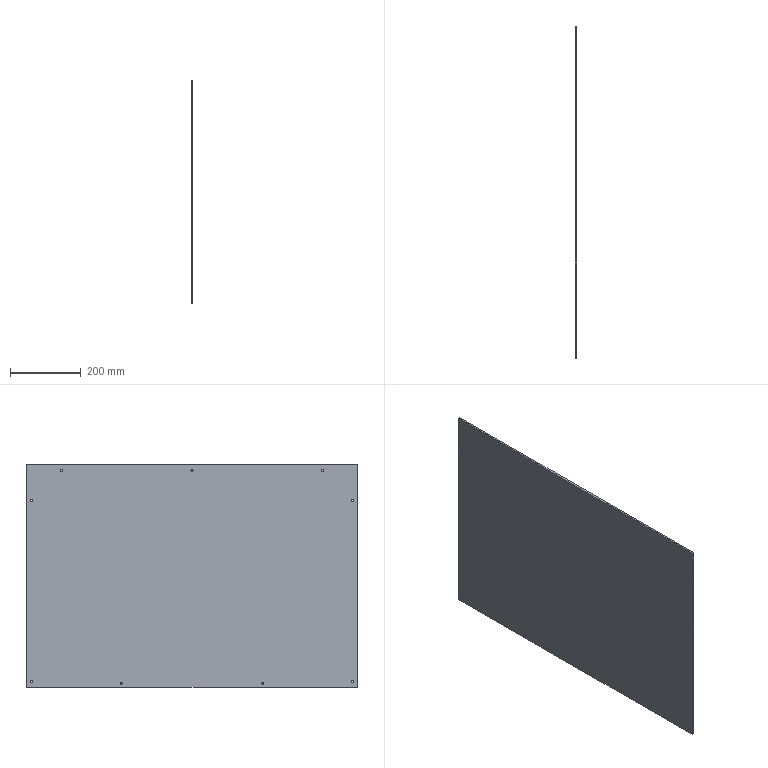Part | SolidWorks | features Chamfer 1, Extrusion 1, ICE 1 | 1 solid | 28 faces | box 5 x 938 x 628 mm | volume 2944038 mm3 | cylinder 18 | plane 10 | commonest cylinder face diameters 6 x18
STEP:
#1=CARTESIAN_POINT('',(5.,-200.,-306.));
#2=VERTEX_POINT('',#1);
#3=CARTESIAN_POINT('',(5.,-200.,-300.));
#4=VERTEX_POINT('',#3);
#5=CARTESIAN_POINT('',(5.,-200.,-303.));
#6=DIRECTION('',(-1.,0.,0.));
#7=DIRECTION('',(0.,0.,1.));
#8=AXIS2_PLACEMENT_3D('',#5,#6,#7);
#9=CIRCLE('',#8,3.);
#10=EDGE_CURVE('',#2,#4,#9,.T.);
#11=ORIENTED_EDGE('',*,*,#10,.F.);
#12=CARTESIAN_POINT('',(0.,-200.,-306.));
#13=VERTEX_POINT('',#12);
#14=CARTESIAN_POINT('',(5.,-200.,-306.));
#15=DIRECTION('',(-1.,0.,0.));
#16=VECTOR('',#15,1000.);
#17=LINE('',#14,#16);
#18=EDGE_CURVE('',#2,#13,#17,.T.);
#19=ORIENTED_EDGE('',*,*,#18,.T.);
#20=CARTESIAN_POINT('',(0.,-200.,-300.));
#21=VERTEX_POINT('',#20);
#22=CARTESIAN_POINT('',(0.,-200.,-303.));
#23=DIRECTION('',(-1.,0.,0.));
#24=DIRECTION('',(0.,0.,1.));
#25=AXIS2_PLACEMENT_3D('',#22,#23,#24);
#26=CIRCLE('',#25,3.);
#27=EDGE_CURVE('',#13,#21,#26,.T.);
#28=ORIENTED_EDGE('',*,*,#27,.T.);
#29=CARTESIAN_POINT('',(5.,-200.,-300.));
#30=DIRECTION('',(-1.,0.,0.));
#31=VECTOR('',#30,1000.);
#32=LINE('',#29,#31);
#33=EDGE_CURVE('',#4,#21,#32,.T.);
#34=ORIENTED_EDGE('',*,*,#33,.F.);
#35=EDGE_LOOP('',(#11,#19,#28,#34));
#36=FACE_OUTER_BOUND('',#35,.T.);
#37=CARTESIAN_POINT('',(5.,-200.,-303.));
#38=DIRECTION('',(-1.,0.,0.));
#39=DIRECTION('',(0.,0.,1.));
#40=AXIS2_PLACEMENT_3D('',#37,#38,#39);
#41=CYLINDRICAL_SURFACE('',#40,3.);
#42=ADVANCED_FACE('',(#36),#41,.F.);
#43=CARTESIAN_POINT('',(5.,200.,-306.));
#44=VERTEX_POINT('',#43);
#45=CARTESIAN_POINT('',(5.,200.,-300.));
#46=VERTEX_POINT('',#45);
#47=CARTESIAN_POINT('',(5.,200.,-303.));
#48=DIRECTION('',(-1.,0.,0.));
#49=DIRECTION('',(0.,0.,1.));
#50=AXIS2_PLACEMENT_3D('',#47,#48,#49);
#51=CIRCLE('',#50,3.);
#52=EDGE_CURVE('',#44,#46,#51,.T.);
#53=ORIENTED_EDGE('',*,*,#52,.F.);
#54=CARTESIAN_POINT('',(0.,200.,-306.));
#55=VERTEX_POINT('',#54);
#56=CARTESIAN_POINT('',(5.,200.,-306.));
#57=DIRECTION('',(-1.,0.,0.));
#58=VECTOR('',#57,1000.);
#59=LINE('',#56,#58);
#60=EDGE_CURVE('',#44,#55,#59,.T.);
#61=ORIENTED_EDGE('',*,*,#60,.T.);
#62=CARTESIAN_POINT('',(0.,200.,-300.));
#63=VERTEX_POINT('',#62);
#64=CARTESIAN_POINT('',(0.,200.,-303.));
#65=DIRECTION('',(-1.,0.,0.));
#66=DIRECTION('',(0.,0.,1.));
#67=AXIS2_PLACEMENT_3D('',#64,#65,#66);
#68=CIRCLE('',#67,3.);
#69=EDGE_CURVE('',#55,#63,#68,.T.);
#70=ORIENTED_EDGE('',*,*,#69,.T.);
#71=CARTESIAN_POINT('',(5.,200.,-300.));
#72=DIRECTION('',(-1.,0.,0.));
#73=VECTOR('',#72,1000.);
#74=LINE('',#71,#73);
#75=EDGE_CURVE('',#46,#63,#74,.T.);
#76=ORIENTED_EDGE('',*,*,#75,.F.);
#77=EDGE_LOOP('',(#53,#61,#70,#76));
#78=FACE_OUTER_BOUND('',#77,.T.);
#79=CARTESIAN_POINT('',(5.,200.,-303.));
#80=DIRECTION('',(-1.,0.,0.));
#81=DIRECTION('',(0.,0.,1.));
#82=AXIS2_PLACEMENT_3D('',#79,#80,#81);
#83=CYLINDRICAL_SURFACE('',#82,3.);
#84=ADVANCED_FACE('',(#78),#83,.F.);
#85=CARTESIAN_POINT('',(5.,0.,296.));
#86=VERTEX_POINT('',#85);
#87=CARTESIAN_POINT('',(5.,0.,302.));
#88=VERTEX_POINT('',#87);
#89=CARTESIAN_POINT('',(5.,0.,299.));
#90=DIRECTION('',(-1.,0.,0.));
#91=DIRECTION('',(0.,0.,1.));
#92=AXIS2_PLACEMENT_3D('',#89,#90,#91);
#93=CIRCLE('',#92,3.);
#94=EDGE_CURVE('',#86,#88,#93,.T.);
#95=ORIENTED_EDGE('',*,*,#94,.F.);
#96=CARTESIAN_POINT('',(0.,0.,296.));
#97=VERTEX_POINT('',#96);
#98=CARTESIAN_POINT('',(5.,0.,296.));
#99=DIRECTION('',(-1.,0.,0.));
#100=VECTOR('',#99,1000.);
#101=LINE('',#98,#100);
#102=EDGE_CURVE('',#86,#97,#101,.T.);
#103=ORIENTED_EDGE('',*,*,#102,.T.);
#104=CARTESIAN_POINT('',(0.,0.,302.));
#105=VERTEX_POINT('',#104);
#106=CARTESIAN_POINT('',(0.,0.,299.));
#107=DIRECTION('',(-1.,0.,0.));
#108=DIRECTION('',(0.,0.,1.));
#109=AXIS2_PLACEMENT_3D('',#106,#107,#108);
#110=CIRCLE('',#109,3.);
#111=EDGE_CURVE('',#97,#105,#110,.T.);
#112=ORIENTED_EDGE('',*,*,#111,.T.);
#113=CARTESIAN_POINT('',(5.,0.,302.));
#114=DIRECTION('',(-1.,0.,0.));
#115=VECTOR('',#114,1000.);
#116=LINE('',#113,#115);
#117=EDGE_CURVE('',#88,#105,#116,.T.);
#118=ORIENTED_EDGE('',*,*,#117,.F.);
#119=EDGE_LOOP('',(#95,#103,#112,#118));
#120=FACE_OUTER_BOUND('',#119,.T.);
#121=CARTESIAN_POINT('',(5.,0.,299.));
#122=DIRECTION('',(-1.,0.,0.));
#123=DIRECTION('',(0.,0.,1.));
#124=AXIS2_PLACEMENT_3D('',#121,#122,#123);
#125=CYLINDRICAL_SURFACE('',#124,3.);
#126=ADVANCED_FACE('',(#120),#125,.F.);
#127=CARTESIAN_POINT('',(5.,-454.,211.));
#128=VERTEX_POINT('',#127);
#129=CARTESIAN_POINT('',(5.,-454.,217.));
#130=VERTEX_POINT('',#129);
#131=CARTESIAN_POINT('',(5.,-454.,214.));
#132=DIRECTION('',(-1.,0.,0.));
#133=DIRECTION('',(0.,0.,1.));
#134=AXIS2_PLACEMENT_3D('',#131,#132,#133);
#135=CIRCLE('',#134,3.);
#136=EDGE_CURVE('',#128,#130,#135,.T.);
#137=ORIENTED_EDGE('',*,*,#136,.F.);
#138=CARTESIAN_POINT('',(0.,-454.,211.));
#139=VERTEX_POINT('',#138);
#140=CARTESIAN_POINT('',(5.,-454.,211.));
#141=DIRECTION('',(-1.,0.,0.));
#142=VECTOR('',#141,1000.);
#143=LINE('',#140,#142);
#144=EDGE_CURVE('',#128,#139,#143,.T.);
#145=ORIENTED_EDGE('',*,*,#144,.T.);
#146=CARTESIAN_POINT('',(0.,-454.,217.));
#147=VERTEX_POINT('',#146);
#148=CARTESIAN_POINT('',(0.,-454.,214.));
#149=DIRECTION('',(-1.,0.,0.));
#150=DIRECTION('',(0.,0.,1.));
#151=AXIS2_PLACEMENT_3D('',#148,#149,#150);
#152=CIRCLE('',#151,3.);
#153=EDGE_CURVE('',#139,#147,#152,.T.);
#154=ORIENTED_EDGE('',*,*,#153,.T.);
#155=CARTESIAN_POINT('',(5.,-454.,217.));
#156=DIRECTION('',(-1.,0.,0.));
#157=VECTOR('',#156,1000.);
#158=LINE('',#155,#157);
#159=EDGE_CURVE('',#130,#147,#158,.T.);
#160=ORIENTED_EDGE('',*,*,#159,.F.);
#161=EDGE_LOOP('',(#137,#145,#154,#160));
#162=FACE_OUTER_BOUND('',#161,.T.);
#163=CARTESIAN_POINT('',(5.,-454.,214.));
#164=DIRECTION('',(-1.,0.,0.));
#165=DIRECTION('',(0.,0.,1.));
#166=AXIS2_PLACEMENT_3D('',#163,#164,#165);
#167=CYLINDRICAL_SURFACE('',#166,3.);
#168=ADVANCED_FACE('',(#162),#167,.F.);
#169=CARTESIAN_POINT('',(5.,-369.,296.));
#170=VERTEX_POINT('',#169);
#171=CARTESIAN_POINT('',(5.,-369.,302.));
#172=VERTEX_POINT('',#171);
#173=CARTESIAN_POINT('',(5.,-369.,299.));
#174=DIRECTION('',(-1.,0.,0.));
#175=DIRECTION('',(0.,0.,1.));
#176=AXIS2_PLACEMENT_3D('',#173,#174,#175);
#177=CIRCLE('',#176,3.);
#178=EDGE_CURVE('',#170,#172,#177,.T.);
#179=ORIENTED_EDGE('',*,*,#178,.F.);
#180=CARTESIAN_POINT('',(0.,-369.,296.));
#181=VERTEX_POINT('',#180);
#182=CARTESIAN_POINT('',(5.,-369.,296.));
#183=DIRECTION('',(-1.,0.,0.));
#184=VECTOR('',#183,1000.);
#185=LINE('',#182,#184);
#186=EDGE_CURVE('',#170,#181,#185,.T.);
#187=ORIENTED_EDGE('',*,*,#186,.T.);
#188=CARTESIAN_POINT('',(0.,-369.,302.));
#189=VERTEX_POINT('',#188);
#190=CARTESIAN_POINT('',(0.,-369.,299.));
#191=DIRECTION('',(-1.,0.,0.));
#192=DIRECTION('',(0.,0.,1.));
#193=AXIS2_PLACEMENT_3D('',#190,#191,#192);
#194=CIRCLE('',#193,3.);
#195=EDGE_CURVE('',#181,#189,#194,.T.);
#196=ORIENTED_EDGE('',*,*,#195,.T.);
#197=CARTESIAN_POINT('',(5.,-369.,302.));
#198=DIRECTION('',(-1.,0.,0.));
#199=VECTOR('',#198,1000.);
#200=LINE('',#197,#199);
#201=EDGE_CURVE('',#172,#189,#200,.T.);
#202=ORIENTED_EDGE('',*,*,#201,.F.);
#203=EDGE_LOOP('',(#179,#187,#196,#202));
#204=FACE_OUTER_BOUND('',#203,.T.);
#205=CARTESIAN_POINT('',(5.,-369.,299.));
#206=DIRECTION('',(-1.,0.,0.));
#207=DIRECTION('',(0.,0.,1.));
#208=AXIS2_PLACEMENT_3D('',#205,#206,#207);
#209=CYLINDRICAL_SURFACE('',#208,3.);
#210=ADVANCED_FACE('',(#204),#209,.F.);
#211=CARTESIAN_POINT('',(5.,369.,296.));
#212=VERTEX_POINT('',#211);
#213=CARTESIAN_POINT('',(5.,369.,302.));
#214=VERTEX_POINT('',#213);
#215=CARTESIAN_POINT('',(5.,369.,299.));
#216=DIRECTION('',(-1.,0.,0.));
#217=DIRECTION('',(0.,0.,1.));
#218=AXIS2_PLACEMENT_3D('',#215,#216,#217);
#219=CIRCLE('',#218,3.);
#220=EDGE_CURVE('',#212,#214,#219,.T.);
#221=ORIENTED_EDGE('',*,*,#220,.F.);
#222=CARTESIAN_POINT('',(0.,369.,296.));
#223=VERTEX_POINT('',#222);
#224=CARTESIAN_POINT('',(5.,369.,296.));
#225=DIRECTION('',(-1.,0.,0.));
#226=VECTOR('',#225,1000.);
#227=LINE('',#224,#226);
#228=EDGE_CURVE('',#212,#223,#227,.T.);
#229=ORIENTED_EDGE('',*,*,#228,.T.);
#230=CARTESIAN_POINT('',(0.,369.,302.));
#231=VERTEX_POINT('',#230);
#232=CARTESIAN_POINT('',(0.,369.,299.));
#233=DIRECTION('',(-1.,0.,0.));
#234=DIRECTION('',(0.,0.,1.));
#235=AXIS2_PLACEMENT_3D('',#232,#233,#234);
#236=CIRCLE('',#235,3.);
#237=EDGE_CURVE('',#223,#231,#236,.T.);
#238=ORIENTED_EDGE('',*,*,#237,.T.);
#239=CARTESIAN_POINT('',(5.,369.,302.));
#240=DIRECTION('',(-1.,0.,0.));
#241=VECTOR('',#240,1000.);
#242=LINE('',#239,#241);
#243=EDGE_CURVE('',#214,#231,#242,.T.);
#244=ORIENTED_EDGE('',*,*,#243,.F.);
#245=EDGE_LOOP('',(#221,#229,#238,#244));
#246=FACE_OUTER_BOUND('',#245,.T.);
#247=CARTESIAN_POINT('',(5.,369.,299.));
#248=DIRECTION('',(-1.,0.,0.));
#249=DIRECTION('',(0.,0.,1.));
#250=AXIS2_PLACEMENT_3D('',#247,#248,#249);
#251=CYLINDRICAL_SURFACE('',#250,3.);
#252=ADVANCED_FACE('',(#246),#251,.F.);
#253=CARTESIAN_POINT('',(5.,454.,211.));
#254=VERTEX_POINT('',#253);
#255=CARTESIAN_POINT('',(5.,454.,217.));
#256=VERTEX_POINT('',#255);
#257=CARTESIAN_POINT('',(5.,454.,214.));
#258=DIRECTION('',(-1.,0.,0.));
#259=DIRECTION('',(0.,0.,1.));
#260=AXIS2_PLACEMENT_3D('',#257,#258,#259);
#261=CIRCLE('',#260,3.);
#262=EDGE_CURVE('',#254,#256,#261,.T.);
#263=ORIENTED_EDGE('',*,*,#262,.F.);
#264=CARTESIAN_POINT('',(0.,454.,211.));
#265=VERTEX_POINT('',#264);
#266=CARTESIAN_POINT('',(5.,454.,211.));
#267=DIRECTION('',(-1.,0.,0.));
#268=VECTOR('',#267,1000.);
#269=LINE('',#266,#268);
#270=EDGE_CURVE('',#254,#265,#269,.T.);
#271=ORIENTED_EDGE('',*,*,#270,.T.);
#272=CARTESIAN_POINT('',(0.,454.,217.));
#273=VERTEX_POINT('',#272);
#274=CARTESIAN_POINT('',(0.,454.,214.));
#275=DIRECTION('',(-1.,0.,0.));
#276=DIRECTION('',(0.,0.,1.));
#277=AXIS2_PLACEMENT_3D('',#274,#275,#276);
#278=CIRCLE('',#277,3.);
#279=EDGE_CURVE('',#265,#273,#278,.T.);
#280=ORIENTED_EDGE('',*,*,#279,.T.);
#281=CARTESIAN_POINT('',(5.,454.,217.));
#282=DIRECTION('',(-1.,0.,0.));
#283=VECTOR('',#282,1000.);
#284=LINE('',#281,#283);
#285=EDGE_CURVE('',#256,#273,#284,.T.);
#286=ORIENTED_EDGE('',*,*,#285,.F.);
#287=EDGE_LOOP('',(#263,#271,#280,#286));
#288=FACE_OUTER_BOUND('',#287,.T.);
#289=CARTESIAN_POINT('',(5.,454.,214.));
#290=DIRECTION('',(-1.,0.,0.));
#291=DIRECTION('',(0.,0.,1.));
#292=AXIS2_PLACEMENT_3D('',#289,#290,#291);
#293=CYLINDRICAL_SURFACE('',#292,3.);
#294=ADVANCED_FACE('',(#288),#293,.F.);
#295=CARTESIAN_POINT('',(5.,-454.,-302.));
#296=VERTEX_POINT('',#295);
#297=CARTESIAN_POINT('',(5.,-454.,-296.));
#298=VERTEX_POINT('',#297);
#299=CARTESIAN_POINT('',(5.,-454.,-299.));
#300=DIRECTION('',(-1.,0.,0.));
#301=DIRECTION('',(0.,0.,-1.));
#302=AXIS2_PLACEMENT_3D('',#299,#300,#301);
#303=CIRCLE('',#302,3.);
#304=EDGE_CURVE('',#296,#298,#303,.T.);
#305=ORIENTED_EDGE('',*,*,#304,.F.);
#306=CARTESIAN_POINT('',(0.,-454.,-302.));
#307=VERTEX_POINT('',#306);
#308=CARTESIAN_POINT('',(5.,-454.,-302.));
#309=DIRECTION('',(-1.,0.,0.));
#310=VECTOR('',#309,1000.);
#311=LINE('',#308,#310);
#312=EDGE_CURVE('',#296,#307,#311,.T.);
#313=ORIENTED_EDGE('',*,*,#312,.T.);
#314=CARTESIAN_POINT('',(0.,-454.,-296.));
#315=VERTEX_POINT('',#314);
#316=CARTESIAN_POINT('',(0.,-454.,-299.));
#317=DIRECTION('',(-1.,0.,0.));
#318=DIRECTION('',(0.,0.,-1.));
#319=AXIS2_PLACEMENT_3D('',#316,#317,#318);
#320=CIRCLE('',#319,3.);
#321=EDGE_CURVE('',#307,#315,#320,.T.);
#322=ORIENTED_EDGE('',*,*,#321,.T.);
#323=CARTESIAN_POINT('',(5.,-454.,-296.));
#324=DIRECTION('',(-1.,0.,0.));
#325=VECTOR('',#324,1000.);
#326=LINE('',#323,#325);
#327=EDGE_CURVE('',#298,#315,#326,.T.);
#328=ORIENTED_EDGE('',*,*,#327,.F.);
#329=EDGE_LOOP('',(#305,#313,#322,#328));
#330=FACE_OUTER_BOUND('',#329,.T.);
#331=CARTESIAN_POINT('',(5.,-454.,-299.));
#332=DIRECTION('',(-1.,0.,0.));
#333=DIRECTION('',(0.,0.,1.));
#334=AXIS2_PLACEMENT_3D('',#331,#332,#333);
#335=CYLINDRICAL_SURFACE('',#334,3.);
#336=ADVANCED_FACE('',(#330),#335,.F.);
#337=CARTESIAN_POINT('',(5.,454.,-302.));
#338=VERTEX_POINT('',#337);
#339=CARTESIAN_POINT('',(5.,454.,-296.));
#340=VERTEX_POINT('',#339);
#341=CARTESIAN_POINT('',(5.,454.,-299.));
#342=DIRECTION('',(-1.,0.,0.));
#343=DIRECTION('',(0.,0.,1.));
#344=AXIS2_PLACEMENT_3D('',#341,#342,#343);
#345=CIRCLE('',#344,3.);
#346=EDGE_CURVE('',#338,#340,#345,.T.);
#347=ORIENTED_EDGE('',*,*,#346,.F.);
#348=CARTESIAN_POINT('',(0.,454.,-302.));
#349=VERTEX_POINT('',#348);
#350=CARTESIAN_POINT('',(5.,454.,-302.));
#351=DIRECTION('',(-1.,0.,0.));
#352=VECTOR('',#351,1000.);
#353=LINE('',#350,#352);
#354=EDGE_CURVE('',#338,#349,#353,.T.);
#355=ORIENTED_EDGE('',*,*,#354,.T.);
#356=CARTESIAN_POINT('',(0.,454.,-296.));
#357=VERTEX_POINT('',#356);
#358=CARTESIAN_POINT('',(0.,454.,-299.));
#359=DIRECTION('',(-1.,0.,0.));
#360=DIRECTION('',(0.,0.,1.));
#361=AXIS2_PLACEMENT_3D('',#358,#359,#360);
#362=CIRCLE('',#361,3.);
#363=EDGE_CURVE('',#349,#357,#362,.T.);
#364=ORIENTED_EDGE('',*,*,#363,.T.);
#365=CARTESIAN_POINT('',(5.,454.,-296.));
#366=DIRECTION('',(-1.,0.,0.));
#367=VECTOR('',#366,1000.);
#368=LINE('',#365,#367);
#369=EDGE_CURVE('',#340,#357,#368,.T.);
#370=ORIENTED_EDGE('',*,*,#369,.F.);
#371=EDGE_LOOP('',(#347,#355,#364,#370));
#372=FACE_OUTER_BOUND('',#371,.T.);
#373=CARTESIAN_POINT('',(5.,454.,-299.));
#374=DIRECTION('',(-1.,0.,0.));
#375=DIRECTION('',(0.,0.,1.));
#376=AXIS2_PLACEMENT_3D('',#373,#374,#375);
#377=CYLINDRICAL_SURFACE('',#376,3.);
#378=ADVANCED_FACE('',(#372),#377,.F.);
#379=CARTESIAN_POINT('',(0.,468.,314.));
#380=VERTEX_POINT('',#379);
#381=CARTESIAN_POINT('',(0.,-468.,314.));
#382=VERTEX_POINT('',#381);
#383=CARTESIAN_POINT('',(0.,469.,314.));
#384=DIRECTION('',(0.,-1.,0.));
#385=VECTOR('',#384,1000.);
#386=LINE('',#383,#385);
#387=EDGE_CURVE('',#380,#382,#386,.T.);
#388=ORIENTED_EDGE('',*,*,#387,.T.);
#389=CARTESIAN_POINT('',(5.,-468.,314.));
#390=VERTEX_POINT('',#389);
#391=CARTESIAN_POINT('',(5.,-468.,314.));
#392=DIRECTION('',(1.,0.,0.));
#393=VECTOR('',#392,1000.);
#394=LINE('',#391,#393);
#395=EDGE_CURVE('',#382,#390,#394,.T.);
#396=ORIENTED_EDGE('',*,*,#395,.T.);
#397=CARTESIAN_POINT('',(5.,468.,314.));
#398=VERTEX_POINT('',#397);
#399=CARTESIAN_POINT('',(5.,469.,314.));
#400=DIRECTION('',(0.,-1.,0.));
#401=VECTOR('',#400,1000.);
#402=LINE('',#399,#401);
#403=EDGE_CURVE('',#398,#390,#402,.T.);
#404=ORIENTED_EDGE('',*,*,#403,.F.);
#405=CARTESIAN_POINT('',(5.,468.,314.));
#406=DIRECTION('',(-1.,0.,0.));
#407=VECTOR('',#406,1000.);
#408=LINE('',#405,#407);
#409=EDGE_CURVE('',#398,#380,#408,.T.);
#410=ORIENTED_EDGE('',*,*,#409,.T.);
#411=EDGE_LOOP('',(#388,#396,#404,#410));
#412=FACE_OUTER_BOUND('',#411,.T.);
#413=CARTESIAN_POINT('',(5.,469.,314.));
#414=DIRECTION('',(0.,0.,-1.));
#415=DIRECTION('',(0.,1.,0.));
#416=AXIS2_PLACEMENT_3D('',#413,#414,#415);
#417=PLANE('',#416);
#418=ADVANCED_FACE('',(#412),#417,.F.);
#419=CARTESIAN_POINT('',(0.,-469.,313.));
#420=VERTEX_POINT('',#419);
#421=CARTESIAN_POINT('',(0.,-469.,-313.));
#422=VERTEX_POINT('',#421);
#423=CARTESIAN_POINT('',(0.,-469.,-314.));
#424=DIRECTION('',(0.,0.,-1.));
#425=VECTOR('',#424,1000.);
#426=LINE('',#423,#425);
#427=EDGE_CURVE('',#420,#422,#426,.T.);
#428=ORIENTED_EDGE('',*,*,#427,.T.);
#429=CARTESIAN_POINT('',(5.,-469.,-313.));
#430=VERTEX_POINT('',#429);
#431=CARTESIAN_POINT('',(5.,-469.,-313.));
#432=DIRECTION('',(1.,0.,0.));
#433=VECTOR('',#432,1000.);
#434=LINE('',#431,#433);
#435=EDGE_CURVE('',#422,#430,#434,.T.);
#436=ORIENTED_EDGE('',*,*,#435,.T.);
#437=CARTESIAN_POINT('',(5.,-469.,313.));
#438=VERTEX_POINT('',#437);
#439=CARTESIAN_POINT('',(5.,-469.,-314.));
#440=DIRECTION('',(0.,0.,-1.));
#441=VECTOR('',#440,1000.);
#442=LINE('',#439,#441);
#443=EDGE_CURVE('',#438,#430,#442,.T.);
#444=ORIENTED_EDGE('',*,*,#443,.F.);
#445=CARTESIAN_POINT('',(5.,-469.,313.));
#446=DIRECTION('',(-1.,0.,0.));
#447=VECTOR('',#446,1000.);
#448=LINE('',#445,#447);
#449=EDGE_CURVE('',#438,#420,#448,.T.);
#450=ORIENTED_EDGE('',*,*,#449,.T.);
#451=EDGE_LOOP('',(#428,#436,#444,#450));
#452=FACE_OUTER_BOUND('',#451,.T.);
#453=CARTESIAN_POINT('',(5.,-469.,-314.));
#454=DIRECTION('',(0.,1.,0.));
#455=DIRECTION('',(0.,0.,1.));
#456=AXIS2_PLACEMENT_3D('',#453,#454,#455);
#457=PLANE('',#456);
#458=ADVANCED_FACE('',(#452),#457,.F.);
#459=CARTESIAN_POINT('',(5.,-468.,-314.));
#460=VERTEX_POINT('',#459);
#461=CARTESIAN_POINT('',(5.,468.,-314.));
#462=VERTEX_POINT('',#461);
#463=CARTESIAN_POINT('',(5.,469.,-314.));
#464=DIRECTION('',(0.,1.,0.));
#465=VECTOR('',#464,1000.);
#466=LINE('',#463,#465);
#467=EDGE_CURVE('',#460,#462,#466,.T.);
#468=ORIENTED_EDGE('',*,*,#467,.F.);
#469=CARTESIAN_POINT('',(0.,-468.,-314.));
#470=VERTEX_POINT('',#469);
#471=CARTESIAN_POINT('',(5.,-468.,-314.));
#472=DIRECTION('',(-1.,0.,0.));
#473=VECTOR('',#472,1000.);
#474=LINE('',#471,#473);
#475=EDGE_CURVE('',#460,#470,#474,.T.);
#476=ORIENTED_EDGE('',*,*,#475,.T.);
#477=CARTESIAN_POINT('',(0.,468.,-314.));
#478=VERTEX_POINT('',#477);
#479=CARTESIAN_POINT('',(0.,469.,-314.));
#480=DIRECTION('',(0.,1.,0.));
#481=VECTOR('',#480,1000.);
#482=LINE('',#479,#481);
#483=EDGE_CURVE('',#470,#478,#482,.T.);
#484=ORIENTED_EDGE('',*,*,#483,.T.);
#485=CARTESIAN_POINT('',(5.,468.,-314.));
#486=DIRECTION('',(1.,0.,0.));
#487=VECTOR('',#486,1000.);
#488=LINE('',#485,#487);
#489=EDGE_CURVE('',#478,#462,#488,.T.);
#490=ORIENTED_EDGE('',*,*,#489,.T.);
#491=EDGE_LOOP('',(#468,#476,#484,#490));
#492=FACE_OUTER_BOUND('',#491,.T.);
#493=CARTESIAN_POINT('',(5.,469.,-314.));
#494=DIRECTION('',(0.,0.,1.));
#495=DIRECTION('',(0.,-1.,0.));
#496=AXIS2_PLACEMENT_3D('',#493,#494,#495);
#497=PLANE('',#496);
#498=ADVANCED_FACE('',(#492),#497,.F.);
#499=CARTESIAN_POINT('',(5.,469.,-313.));
#500=VERTEX_POINT('',#499);
#501=CARTESIAN_POINT('',(5.,469.,313.));
#502=VERTEX_POINT('',#501);
#503=CARTESIAN_POINT('',(5.,469.,-314.));
#504=DIRECTION('',(0.,0.,1.));
#505=VECTOR('',#504,1000.);
#506=LINE('',#503,#505);
#507=EDGE_CURVE('',#500,#502,#506,.T.);
#508=ORIENTED_EDGE('',*,*,#507,.F.);
#509=CARTESIAN_POINT('',(0.,469.,-313.));
#510=VERTEX_POINT('',#509);
#511=CARTESIAN_POINT('',(5.,469.,-313.));
#512=DIRECTION('',(-1.,0.,0.));
#513=VECTOR('',#512,1000.);
#514=LINE('',#511,#513);
#515=EDGE_CURVE('',#500,#510,#514,.T.);
#516=ORIENTED_EDGE('',*,*,#515,.T.);
#517=CARTESIAN_POINT('',(0.,469.,313.));
#518=VERTEX_POINT('',#517);
#519=CARTESIAN_POINT('',(0.,469.,-314.));
#520=DIRECTION('',(0.,0.,1.));
#521=VECTOR('',#520,1000.);
#522=LINE('',#519,#521);
#523=EDGE_CURVE('',#510,#518,#522,.T.);
#524=ORIENTED_EDGE('',*,*,#523,.T.);
#525=CARTESIAN_POINT('',(5.,469.,313.));
#526=DIRECTION('',(1.,0.,0.));
#527=VECTOR('',#526,1000.);
#528=LINE('',#525,#527);
#529=EDGE_CURVE('',#518,#502,#528,.T.);
#530=ORIENTED_EDGE('',*,*,#529,.T.);
#531=EDGE_LOOP('',(#508,#516,#524,#530));
#532=FACE_OUTER_BOUND('',#531,.T.);
#533=CARTESIAN_POINT('',(5.,469.,-314.));
#534=DIRECTION('',(0.,-1.,0.));
#535=DIRECTION('',(0.,0.,-1.));
#536=AXIS2_PLACEMENT_3D('',#533,#534,#535);
#537=PLANE('',#536);
#538=ADVANCED_FACE('',(#532),#537,.F.);
#539=CARTESIAN_POINT('',(5.,-200.,-303.));
#540=DIRECTION('',(-1.,0.,0.));
#541=DIRECTION('',(0.,0.,1.));
#542=AXIS2_PLACEMENT_3D('',#539,#540,#541);
#543=CIRCLE('',#542,3.);
#544=EDGE_CURVE('',#4,#2,#543,.T.);
#545=ORIENTED_EDGE('',*,*,#544,.T.);
#546=ORIENTED_EDGE('',*,*,#10,.T.);
#547=EDGE_LOOP('',(#545,#546));
#548=FACE_BOUND('',#547,.T.);
#549=CARTESIAN_POINT('',(5.,200.,-303.));
#550=DIRECTION('',(-1.,0.,0.));
#551=DIRECTION('',(0.,0.,1.));
#552=AXIS2_PLACEMENT_3D('',#549,#550,#551);
#553=CIRCLE('',#552,3.);
#554=EDGE_CURVE('',#46,#44,#553,.T.);
#555=ORIENTED_EDGE('',*,*,#554,.T.);
#556=ORIENTED_EDGE('',*,*,#52,.T.);
#557=EDGE_LOOP('',(#555,#556));
#558=FACE_BOUND('',#557,.T.);
#559=CARTESIAN_POINT('',(5.,0.,299.));
#560=DIRECTION('',(-1.,0.,0.));
#561=DIRECTION('',(0.,0.,1.));
#562=AXIS2_PLACEMENT_3D('',#559,#560,#561);
#563=CIRCLE('',#562,3.);
#564=EDGE_CURVE('',#88,#86,#563,.T.);
#565=ORIENTED_EDGE('',*,*,#564,.T.);
#566=ORIENTED_EDGE('',*,*,#94,.T.);
#567=EDGE_LOOP('',(#565,#566));
#568=FACE_BOUND('',#567,.T.);
#569=CARTESIAN_POINT('',(5.,-454.,214.));
#570=DIRECTION('',(-1.,0.,0.));
#571=DIRECTION('',(0.,0.,1.));
#572=AXIS2_PLACEMENT_3D('',#569,#570,#571);
#573=CIRCLE('',#572,3.);
#574=EDGE_CURVE('',#130,#128,#573,.T.);
#575=ORIENTED_EDGE('',*,*,#574,.T.);
#576=ORIENTED_EDGE('',*,*,#136,.T.);
#577=EDGE_LOOP('',(#575,#576));
#578=FACE_BOUND('',#577,.T.);
#579=CARTESIAN_POINT('',(5.,-369.,299.));
#580=DIRECTION('',(-1.,0.,0.));
#581=DIRECTION('',(0.,0.,1.));
#582=AXIS2_PLACEMENT_3D('',#579,#580,#581);
#583=CIRCLE('',#582,3.);
#584=EDGE_CURVE('',#172,#170,#583,.T.);
#585=ORIENTED_EDGE('',*,*,#584,.T.);
#586=ORIENTED_EDGE('',*,*,#178,.T.);
#587=EDGE_LOOP('',(#585,#586));
#588=FACE_BOUND('',#587,.T.);
#589=CARTESIAN_POINT('',(5.,369.,299.));
#590=DIRECTION('',(-1.,0.,0.));
#591=DIRECTION('',(0.,0.,1.));
#592=AXIS2_PLACEMENT_3D('',#589,#590,#591);
#593=CIRCLE('',#592,3.);
#594=EDGE_CURVE('',#214,#212,#593,.T.);
#595=ORIENTED_EDGE('',*,*,#594,.T.);
#596=ORIENTED_EDGE('',*,*,#220,.T.);
#597=EDGE_LOOP('',(#595,#596));
#598=FACE_BOUND('',#597,.T.);
#599=CARTESIAN_POINT('',(5.,454.,214.));
#600=DIRECTION('',(-1.,0.,0.));
#601=DIRECTION('',(0.,0.,1.));
#602=AXIS2_PLACEMENT_3D('',#599,#600,#601);
#603=CIRCLE('',#602,3.);
#604=EDGE_CURVE('',#256,#254,#603,.T.);
#605=ORIENTED_EDGE('',*,*,#604,.T.);
#606=ORIENTED_EDGE('',*,*,#262,.T.);
#607=EDGE_LOOP('',(#605,#606));
#608=FACE_BOUND('',#607,.T.);
#609=CARTESIAN_POINT('',(5.,-454.,-299.));
#610=DIRECTION('',(-1.,0.,0.));
#611=DIRECTION('',(0.,0.,-1.));
#612=AXIS2_PLACEMENT_3D('',#609,#610,#611);
#613=CIRCLE('',#612,3.);
#614=EDGE_CURVE('',#298,#296,#613,.T.);
#615=ORIENTED_EDGE('',*,*,#614,.T.);
#616=ORIENTED_EDGE('',*,*,#304,.T.);
#617=EDGE_LOOP('',(#615,#616));
#618=FACE_BOUND('',#617,.T.);
#619=CARTESIAN_POINT('',(5.,454.,-299.));
#620=DIRECTION('',(-1.,0.,0.));
#621=DIRECTION('',(0.,0.,1.));
#622=AXIS2_PLACEMENT_3D('',#619,#620,#621);
#623=CIRCLE('',#622,3.);
#624=EDGE_CURVE('',#340,#338,#623,.T.);
#625=ORIENTED_EDGE('',*,*,#624,.T.);
#626=ORIENTED_EDGE('',*,*,#346,.T.);
#627=EDGE_LOOP('',(#625,#626));
#628=FACE_BOUND('',#627,.T.);
#629=ORIENTED_EDGE('',*,*,#443,.T.);
#630=CARTESIAN_POINT('',(5.,-468.,-314.));
#631=DIRECTION('',(0.,0.7071,-0.7071));
#632=VECTOR('',#631,1000.);
#633=LINE('',#630,#632);
#634=EDGE_CURVE('',#430,#460,#633,.T.);
#635=ORIENTED_EDGE('',*,*,#634,.T.);
#636=ORIENTED_EDGE('',*,*,#467,.T.);
#637=CARTESIAN_POINT('',(5.,469.,-313.));
#638=DIRECTION('',(0.,0.7071,0.7071));
#639=VECTOR('',#638,1000.);
#640=LINE('',#637,#639);
#641=EDGE_CURVE('',#462,#500,#640,.T.);
#642=ORIENTED_EDGE('',*,*,#641,.T.);
#643=ORIENTED_EDGE('',*,*,#507,.T.);
#644=CARTESIAN_POINT('',(5.,468.,314.));
#645=DIRECTION('',(0.,-0.7071,0.7071));
#646=VECTOR('',#645,1000.);
#647=LINE('',#644,#646);
#648=EDGE_CURVE('',#502,#398,#647,.T.);
#649=ORIENTED_EDGE('',*,*,#648,.T.);
#650=ORIENTED_EDGE('',*,*,#403,.T.);
#651=CARTESIAN_POINT('',(5.,-469.,313.));
#652=DIRECTION('',(0.,-0.7071,-0.7071));
#653=VECTOR('',#652,1000.);
#654=LINE('',#651,#653);
#655=EDGE_CURVE('',#390,#438,#654,.T.);
#656=ORIENTED_EDGE('',*,*,#655,.T.);
#657=EDGE_LOOP('',(#629,#635,#636,#642,#643,#649,#650,#656));
#658=FACE_OUTER_BOUND('',#657,.T.);
#659=CARTESIAN_POINT('',(5.,-469.,314.));
#660=DIRECTION('',(-1.,0.,0.));
#661=DIRECTION('',(0.,0.,1.));
#662=AXIS2_PLACEMENT_3D('',#659,#660,#661);
#663=PLANE('',#662);
#664=ADVANCED_FACE('',(#548,#558,#568,#578,#588,#598,#608,#618,#628,#658),#663,.F.);
#665=CARTESIAN_POINT('',(0.,-200.,-303.));
#666=DIRECTION('',(-1.,0.,0.));
#667=DIRECTION('',(0.,0.,1.));
#668=AXIS2_PLACEMENT_3D('',#665,#666,#667);
#669=CIRCLE('',#668,3.);
#670=EDGE_CURVE('',#21,#13,#669,.T.);
#671=ORIENTED_EDGE('',*,*,#670,.F.);
#672=ORIENTED_EDGE('',*,*,#27,.F.);
#673=EDGE_LOOP('',(#671,#672));
#674=FACE_BOUND('',#673,.T.);
#675=CARTESIAN_POINT('',(0.,200.,-303.));
#676=DIRECTION('',(-1.,0.,0.));
#677=DIRECTION('',(0.,0.,1.));
#678=AXIS2_PLACEMENT_3D('',#675,#676,#677);
#679=CIRCLE('',#678,3.);
#680=EDGE_CURVE('',#63,#55,#679,.T.);
#681=ORIENTED_EDGE('',*,*,#680,.F.);
#682=ORIENTED_EDGE('',*,*,#69,.F.);
#683=EDGE_LOOP('',(#681,#682));
#684=FACE_BOUND('',#683,.T.);
#685=CARTESIAN_POINT('',(0.,0.,299.));
#686=DIRECTION('',(-1.,0.,0.));
#687=DIRECTION('',(0.,0.,1.));
#688=AXIS2_PLACEMENT_3D('',#685,#686,#687);
#689=CIRCLE('',#688,3.);
#690=EDGE_CURVE('',#105,#97,#689,.T.);
#691=ORIENTED_EDGE('',*,*,#690,.F.);
#692=ORIENTED_EDGE('',*,*,#111,.F.);
#693=EDGE_LOOP('',(#691,#692));
#694=FACE_BOUND('',#693,.T.);
#695=CARTESIAN_POINT('',(0.,-454.,214.));
#696=DIRECTION('',(-1.,0.,0.));
#697=DIRECTION('',(0.,0.,1.));
#698=AXIS2_PLACEMENT_3D('',#695,#696,#697);
#699=CIRCLE('',#698,3.);
#700=EDGE_CURVE('',#147,#139,#699,.T.);
#701=ORIENTED_EDGE('',*,*,#700,.F.);
#702=ORIENTED_EDGE('',*,*,#153,.F.);
#703=EDGE_LOOP('',(#701,#702));
#704=FACE_BOUND('',#703,.T.);
#705=CARTESIAN_POINT('',(0.,-369.,299.));
#706=DIRECTION('',(-1.,0.,0.));
#707=DIRECTION('',(0.,0.,1.));
#708=AXIS2_PLACEMENT_3D('',#705,#706,#707);
#709=CIRCLE('',#708,3.);
#710=EDGE_CURVE('',#189,#181,#709,.T.);
#711=ORIENTED_EDGE('',*,*,#710,.F.);
#712=ORIENTED_EDGE('',*,*,#195,.F.);
#713=EDGE_LOOP('',(#711,#712));
#714=FACE_BOUND('',#713,.T.);
#715=CARTESIAN_POINT('',(0.,369.,299.));
#716=DIRECTION('',(-1.,0.,0.));
#717=DIRECTION('',(0.,0.,1.));
#718=AXIS2_PLACEMENT_3D('',#715,#716,#717);
#719=CIRCLE('',#718,3.);
#720=EDGE_CURVE('',#231,#223,#719,.T.);
#721=ORIENTED_EDGE('',*,*,#720,.F.);
#722=ORIENTED_EDGE('',*,*,#237,.F.);
#723=EDGE_LOOP('',(#721,#722));
#724=FACE_BOUND('',#723,.T.);
#725=CARTESIAN_POINT('',(0.,454.,214.));
#726=DIRECTION('',(-1.,0.,0.));
#727=DIRECTION('',(0.,0.,1.));
#728=AXIS2_PLACEMENT_3D('',#725,#726,#727);
#729=CIRCLE('',#728,3.);
#730=EDGE_CURVE('',#273,#265,#729,.T.);
#731=ORIENTED_EDGE('',*,*,#730,.F.);
#732=ORIENTED_EDGE('',*,*,#279,.F.);
#733=EDGE_LOOP('',(#731,#732));
#734=FACE_BOUND('',#733,.T.);
#735=CARTESIAN_POINT('',(0.,-454.,-299.));
#736=DIRECTION('',(-1.,0.,0.));
#737=DIRECTION('',(0.,0.,-1.));
#738=AXIS2_PLACEMENT_3D('',#735,#736,#737);
#739=CIRCLE('',#738,3.);
#740=EDGE_CURVE('',#315,#307,#739,.T.);
#741=ORIENTED_EDGE('',*,*,#740,.F.);
#742=ORIENTED_EDGE('',*,*,#321,.F.);
#743=EDGE_LOOP('',(#741,#742));
#744=FACE_BOUND('',#743,.T.);
#745=CARTESIAN_POINT('',(0.,454.,-299.));
#746=DIRECTION('',(-1.,0.,0.));
#747=DIRECTION('',(0.,0.,1.));
#748=AXIS2_PLACEMENT_3D('',#745,#746,#747);
#749=CIRCLE('',#748,3.);
#750=EDGE_CURVE('',#357,#349,#749,.T.);
#751=ORIENTED_EDGE('',*,*,#750,.F.);
#752=ORIENTED_EDGE('',*,*,#363,.F.);
#753=EDGE_LOOP('',(#751,#752));
#754=FACE_BOUND('',#753,.T.);
#755=ORIENTED_EDGE('',*,*,#483,.F.);
#756=CARTESIAN_POINT('',(0.,-782.5,0.5));
#757=DIRECTION('',(0.,-0.7071,0.7071));
#758=VECTOR('',#757,1000.);
#759=LINE('',#756,#758);
#760=EDGE_CURVE('',#470,#422,#759,.T.);
#761=ORIENTED_EDGE('',*,*,#760,.T.);
#762=ORIENTED_EDGE('',*,*,#427,.F.);
#763=CARTESIAN_POINT('',(0.,-468.5,313.5));
#764=DIRECTION('',(0.,0.7071,0.7071));
#765=VECTOR('',#764,1000.);
#766=LINE('',#763,#765);
#767=EDGE_CURVE('',#420,#382,#766,.T.);
#768=ORIENTED_EDGE('',*,*,#767,.T.);
#769=ORIENTED_EDGE('',*,*,#387,.F.);
#770=CARTESIAN_POINT('',(0.,-0.5,782.5));
#771=DIRECTION('',(0.,0.7071,-0.7071));
#772=VECTOR('',#771,1000.);
#773=LINE('',#770,#772);
#774=EDGE_CURVE('',#380,#518,#773,.T.);
#775=ORIENTED_EDGE('',*,*,#774,.T.);
#776=ORIENTED_EDGE('',*,*,#523,.F.);
#777=CARTESIAN_POINT('',(0.,313.5,-468.5));
#778=DIRECTION('',(0.,-0.7071,-0.7071));
#779=VECTOR('',#778,1000.);
#780=LINE('',#777,#779);
#781=EDGE_CURVE('',#510,#478,#780,.T.);
#782=ORIENTED_EDGE('',*,*,#781,.T.);
#783=EDGE_LOOP('',(#755,#761,#762,#768,#769,#775,#776,#782));
#784=FACE_OUTER_BOUND('',#783,.T.);
#785=CARTESIAN_POINT('',(0.,-469.,314.));
#786=DIRECTION('',(-1.,0.,0.));
#787=DIRECTION('',(0.,0.,1.));
#788=AXIS2_PLACEMENT_3D('',#785,#786,#787);
#789=PLANE('',#788);
#790=ADVANCED_FACE('',(#674,#684,#694,#704,#714,#724,#734,#744,#754,#784),#789,.T.);
#791=ORIENTED_EDGE('',*,*,#634,.F.);
#792=ORIENTED_EDGE('',*,*,#435,.F.);
#793=ORIENTED_EDGE('',*,*,#760,.F.);
#794=ORIENTED_EDGE('',*,*,#475,.F.);
#795=EDGE_LOOP('',(#791,#792,#793,#794));
#796=FACE_OUTER_BOUND('',#795,.T.);
#797=CARTESIAN_POINT('',(5.,-468.,-314.));
#798=DIRECTION('',(0.,0.7071,0.7071));
#799=DIRECTION('',(0.,-0.7071,0.7071));
#800=AXIS2_PLACEMENT_3D('',#797,#798,#799);
#801=PLANE('',#800);
#802=ADVANCED_FACE('',(#796),#801,.F.);
#803=ORIENTED_EDGE('',*,*,#655,.F.);
#804=ORIENTED_EDGE('',*,*,#395,.F.);
#805=ORIENTED_EDGE('',*,*,#767,.F.);
#806=ORIENTED_EDGE('',*,*,#449,.F.);
#807=EDGE_LOOP('',(#803,#804,#805,#806));
#808=FACE_OUTER_BOUND('',#807,.T.);
#809=CARTESIAN_POINT('',(5.,-469.,313.));
#810=DIRECTION('',(0.,0.7071,-0.7071));
#811=DIRECTION('',(0.,0.7071,0.7071));
#812=AXIS2_PLACEMENT_3D('',#809,#810,#811);
#813=PLANE('',#812);
#814=ADVANCED_FACE('',(#808),#813,.F.);
#815=ORIENTED_EDGE('',*,*,#641,.F.);
#816=ORIENTED_EDGE('',*,*,#489,.F.);
#817=ORIENTED_EDGE('',*,*,#781,.F.);
#818=ORIENTED_EDGE('',*,*,#515,.F.);
#819=EDGE_LOOP('',(#815,#816,#817,#818));
#820=FACE_OUTER_BOUND('',#819,.T.);
#821=CARTESIAN_POINT('',(5.,469.,-313.));
#822=DIRECTION('',(0.,-0.7071,0.7071));
#823=DIRECTION('',(0.,-0.7071,-0.7071));
#824=AXIS2_PLACEMENT_3D('',#821,#822,#823);
#825=PLANE('',#824);
#826=ADVANCED_FACE('',(#820),#825,.F.);
#827=ORIENTED_EDGE('',*,*,#648,.F.);
#828=ORIENTED_EDGE('',*,*,#529,.F.);
#829=ORIENTED_EDGE('',*,*,#774,.F.);
#830=ORIENTED_EDGE('',*,*,#409,.F.);
#831=EDGE_LOOP('',(#827,#828,#829,#830));
#832=FACE_OUTER_BOUND('',#831,.T.);
#833=CARTESIAN_POINT('',(5.,468.,314.));
#834=DIRECTION('',(0.,-0.7071,-0.7071));
#835=DIRECTION('',(0.,0.7071,-0.7071));
#836=AXIS2_PLACEMENT_3D('',#833,#834,#835);
#837=PLANE('',#836);
#838=ADVANCED_FACE('',(#832),#837,.F.);
#839=ORIENTED_EDGE('',*,*,#354,.F.);
#840=ORIENTED_EDGE('',*,*,#624,.F.);
#841=ORIENTED_EDGE('',*,*,#369,.T.);
#842=ORIENTED_EDGE('',*,*,#750,.T.);
#843=EDGE_LOOP('',(#839,#840,#841,#842));
#844=FACE_OUTER_BOUND('',#843,.T.);
#845=CARTESIAN_POINT('',(5.,454.,-299.));
#846=DIRECTION('',(-1.,0.,0.));
#847=DIRECTION('',(0.,0.,1.));
#848=AXIS2_PLACEMENT_3D('',#845,#846,#847);
#849=CYLINDRICAL_SURFACE('',#848,3.);
#850=ADVANCED_FACE('',(#844),#849,.F.);
#851=ORIENTED_EDGE('',*,*,#312,.F.);
#852=ORIENTED_EDGE('',*,*,#614,.F.);
#853=ORIENTED_EDGE('',*,*,#327,.T.);
#854=ORIENTED_EDGE('',*,*,#740,.T.);
#855=EDGE_LOOP('',(#851,#852,#853,#854));
#856=FACE_OUTER_BOUND('',#855,.T.);
#857=CARTESIAN_POINT('',(5.,-454.,-299.));
#858=DIRECTION('',(-1.,0.,0.));
#859=DIRECTION('',(0.,0.,1.));
#860=AXIS2_PLACEMENT_3D('',#857,#858,#859);
#861=CYLINDRICAL_SURFACE('',#860,3.);
#862=ADVANCED_FACE('',(#856),#861,.F.);
#863=ORIENTED_EDGE('',*,*,#270,.F.);
#864=ORIENTED_EDGE('',*,*,#604,.F.);
#865=ORIENTED_EDGE('',*,*,#285,.T.);
#866=ORIENTED_EDGE('',*,*,#730,.T.);
#867=EDGE_LOOP('',(#863,#864,#865,#866));
#868=FACE_OUTER_BOUND('',#867,.T.);
#869=CARTESIAN_POINT('',(5.,454.,214.));
#870=DIRECTION('',(-1.,0.,0.));
#871=DIRECTION('',(0.,0.,1.));
#872=AXIS2_PLACEMENT_3D('',#869,#870,#871);
#873=CYLINDRICAL_SURFACE('',#872,3.);
#874=ADVANCED_FACE('',(#868),#873,.F.);
#875=ORIENTED_EDGE('',*,*,#228,.F.);
#876=ORIENTED_EDGE('',*,*,#594,.F.);
#877=ORIENTED_EDGE('',*,*,#243,.T.);
#878=ORIENTED_EDGE('',*,*,#720,.T.);
#879=EDGE_LOOP('',(#875,#876,#877,#878));
#880=FACE_OUTER_BOUND('',#879,.T.);
#881=CARTESIAN_POINT('',(5.,369.,299.));
#882=DIRECTION('',(-1.,0.,0.));
#883=DIRECTION('',(0.,0.,1.));
#884=AXIS2_PLACEMENT_3D('',#881,#882,#883);
#885=CYLINDRICAL_SURFACE('',#884,3.);
#886=ADVANCED_FACE('',(#880),#885,.F.);
#887=ORIENTED_EDGE('',*,*,#186,.F.);
#888=ORIENTED_EDGE('',*,*,#584,.F.);
#889=ORIENTED_EDGE('',*,*,#201,.T.);
#890=ORIENTED_EDGE('',*,*,#710,.T.);
#891=EDGE_LOOP('',(#887,#888,#889,#890));
#892=FACE_OUTER_BOUND('',#891,.T.);
#893=CARTESIAN_POINT('',(5.,-369.,299.));
#894=DIRECTION('',(-1.,0.,0.));
#895=DIRECTION('',(0.,0.,1.));
#896=AXIS2_PLACEMENT_3D('',#893,#894,#895);
#897=CYLINDRICAL_SURFACE('',#896,3.);
#898=ADVANCED_FACE('',(#892),#897,.F.);
#899=ORIENTED_EDGE('',*,*,#144,.F.);
#900=ORIENTED_EDGE('',*,*,#574,.F.);
#901=ORIENTED_EDGE('',*,*,#159,.T.);
#902=ORIENTED_EDGE('',*,*,#700,.T.);
#903=EDGE_LOOP('',(#899,#900,#901,#902));
#904=FACE_OUTER_BOUND('',#903,.T.);
#905=CARTESIAN_POINT('',(5.,-454.,214.));
#906=DIRECTION('',(-1.,0.,0.));
#907=DIRECTION('',(0.,0.,1.));
#908=AXIS2_PLACEMENT_3D('',#905,#906,#907);
#909=CYLINDRICAL_SURFACE('',#908,3.);
#910=ADVANCED_FACE('',(#904),#909,.F.);
#911=ORIENTED_EDGE('',*,*,#102,.F.);
#912=ORIENTED_EDGE('',*,*,#564,.F.);
#913=ORIENTED_EDGE('',*,*,#117,.T.);
#914=ORIENTED_EDGE('',*,*,#690,.T.);
#915=EDGE_LOOP('',(#911,#912,#913,#914));
#916=FACE_OUTER_BOUND('',#915,.T.);
#917=CARTESIAN_POINT('',(5.,0.,299.));
#918=DIRECTION('',(-1.,0.,0.));
#919=DIRECTION('',(0.,0.,1.));
#920=AXIS2_PLACEMENT_3D('',#917,#918,#919);
#921=CYLINDRICAL_SURFACE('',#920,3.);
#922=ADVANCED_FACE('',(#916),#921,.F.);
#923=ORIENTED_EDGE('',*,*,#60,.F.);
#924=ORIENTED_EDGE('',*,*,#554,.F.);
#925=ORIENTED_EDGE('',*,*,#75,.T.);
#926=ORIENTED_EDGE('',*,*,#680,.T.);
#927=EDGE_LOOP('',(#923,#924,#925,#926));
#928=FACE_OUTER_BOUND('',#927,.T.);
#929=CARTESIAN_POINT('',(5.,200.,-303.));
#930=DIRECTION('',(-1.,0.,0.));
#931=DIRECTION('',(0.,0.,1.));
#932=AXIS2_PLACEMENT_3D('',#929,#930,#931);
#933=CYLINDRICAL_SURFACE('',#932,3.);
#934=ADVANCED_FACE('',(#928),#933,.F.);
#935=ORIENTED_EDGE('',*,*,#18,.F.);
#936=ORIENTED_EDGE('',*,*,#544,.F.);
#937=ORIENTED_EDGE('',*,*,#33,.T.);
#938=ORIENTED_EDGE('',*,*,#670,.T.);
#939=EDGE_LOOP('',(#935,#936,#937,#938));
#940=FACE_OUTER_BOUND('',#939,.T.);
#941=CARTESIAN_POINT('',(5.,-200.,-303.));
#942=DIRECTION('',(-1.,0.,0.));
#943=DIRECTION('',(0.,0.,1.));
#944=AXIS2_PLACEMENT_3D('',#941,#942,#943);
#945=CYLINDRICAL_SURFACE('',#944,3.);
#946=ADVANCED_FACE('',(#940),#945,.F.);
#947=CLOSED_SHELL('',(#42,#84,#126,#168,#210,#252,#294,#336,#378,#418,#458,#498,#538,#664,#790,#802,#814,#826,#838,#850,#862,#874,#886,#898,#910,#922,#934,#946));
#948=MANIFOLD_SOLID_BREP('',#947);
#949=CARTESIAN_POINT('',(0.,0.,0.));
#950=DIRECTION('',(0.,0.,1.));
#951=DIRECTION('',(1.,0.,0.));
#952=AXIS2_PLACEMENT_3D('',#949,#950,#951);
#953=(LENGTH_UNIT()NAMED_UNIT(*)SI_UNIT(.MILLI.,.METRE.));
#954=UNCERTAINTY_MEASURE_WITH_UNIT(LENGTH_MEASURE(0.00001),#953,'','');
#955=(NAMED_UNIT(*)PLANE_ANGLE_UNIT()SI_UNIT($,.RADIAN.));
#956=(NAMED_UNIT(*)SI_UNIT($,.STERADIAN.)SOLID_ANGLE_UNIT());
#957=(GEOMETRIC_REPRESENTATION_CONTEXT(3)GLOBAL_UNCERTAINTY_ASSIGNED_CONTEXT((#954))GLOBAL_UNIT_ASSIGNED_CONTEXT((#953,#955,#956))REPRESENTATION_CONTEXT('',''));
#958=ADVANCED_BREP_SHAPE_REPRESENTATION('',(#948,#952),#957);